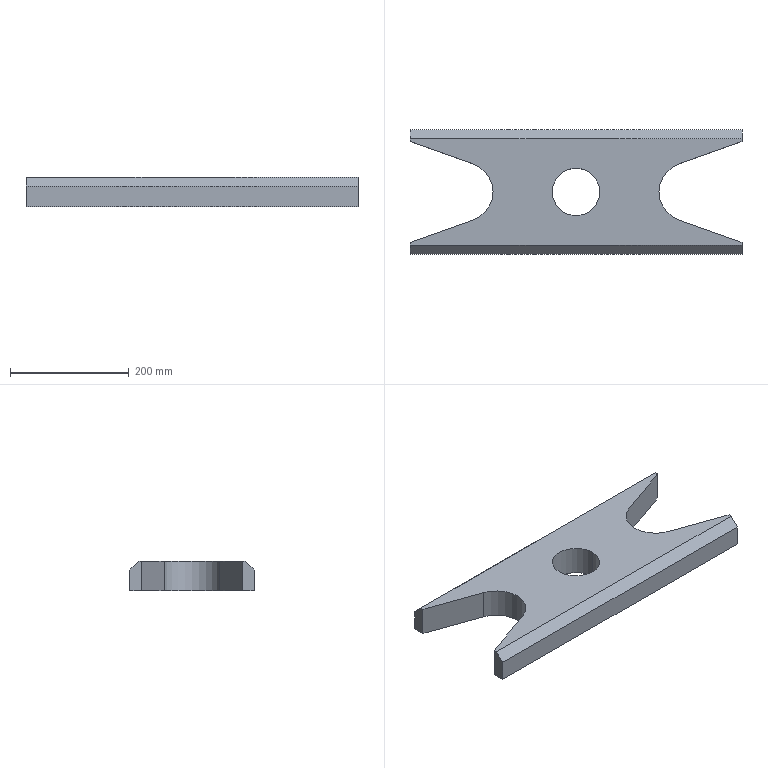Part | SolidWorks | features Chamfer 1, Extrusion 1 | 1 solid | 19 faces | box 560 x 210 x 50 mm | volume 3864002 mm3 | plane 14 | cylinder 5 | commonest cylinder face diameters 100 x3 80 x2
STEP:
#1=CARTESIAN_POINT('',(-40.,0.,25.));
#2=VERTEX_POINT('',#1);
#3=CARTESIAN_POINT('',(40.,0.,25.));
#4=VERTEX_POINT('',#3);
#5=CARTESIAN_POINT('',(0.,0.,25.));
#6=DIRECTION('',(0.,0.,1.));
#7=DIRECTION('',(1.,0.,0.));
#8=AXIS2_PLACEMENT_3D('',#5,#6,#7);
#9=CIRCLE('',#8,40.);
#10=EDGE_CURVE('',#2,#4,#9,.T.);
#11=ORIENTED_EDGE('',*,*,#10,.T.);
#12=CARTESIAN_POINT('',(40.,0.,-25.));
#13=VERTEX_POINT('',#12);
#14=CARTESIAN_POINT('',(40.,0.,25.));
#15=DIRECTION('',(0.,0.,-1.));
#16=VECTOR('',#15,1000.);
#17=LINE('',#14,#16);
#18=EDGE_CURVE('',#4,#13,#17,.T.);
#19=ORIENTED_EDGE('',*,*,#18,.T.);
#20=CARTESIAN_POINT('',(-40.,0.,-25.));
#21=VERTEX_POINT('',#20);
#22=CARTESIAN_POINT('',(0.,0.,-25.));
#23=DIRECTION('',(0.,0.,1.));
#24=DIRECTION('',(1.,0.,0.));
#25=AXIS2_PLACEMENT_3D('',#22,#23,#24);
#26=CIRCLE('',#25,40.);
#27=EDGE_CURVE('',#21,#13,#26,.T.);
#28=ORIENTED_EDGE('',*,*,#27,.F.);
#29=CARTESIAN_POINT('',(-40.,0.,25.));
#30=DIRECTION('',(0.,0.,-1.));
#31=VECTOR('',#30,1000.);
#32=LINE('',#29,#31);
#33=EDGE_CURVE('',#2,#21,#32,.T.);
#34=ORIENTED_EDGE('',*,*,#33,.F.);
#35=EDGE_LOOP('',(#11,#19,#28,#34));
#36=FACE_OUTER_BOUND('',#35,.T.);
#37=CARTESIAN_POINT('',(0.,0.,25.));
#38=DIRECTION('',(0.,0.,-1.));
#39=DIRECTION('',(-1.,0.,0.));
#40=AXIS2_PLACEMENT_3D('',#37,#38,#39);
#41=CYLINDRICAL_SURFACE('',#40,40.);
#42=ADVANCED_FACE('',(#36),#41,.F.);
#43=CARTESIAN_POINT('',(140.,0.,25.));
#44=VERTEX_POINT('',#43);
#45=CARTESIAN_POINT('',(173.276,47.12,25.));
#46=VERTEX_POINT('',#45);
#47=CARTESIAN_POINT('',(190.,0.,25.));
#48=DIRECTION('',(0.,0.,-1.));
#49=DIRECTION('',(1.,0.,0.));
#50=AXIS2_PLACEMENT_3D('',#47,#48,#49);
#51=CIRCLE('',#50,50.);
#52=EDGE_CURVE('',#44,#46,#51,.T.);
#53=ORIENTED_EDGE('',*,*,#52,.F.);
#54=CARTESIAN_POINT('',(140.,0.,-25.));
#55=VERTEX_POINT('',#54);
#56=CARTESIAN_POINT('',(140.,0.,25.));
#57=DIRECTION('',(0.,0.,-1.));
#58=VECTOR('',#57,1000.);
#59=LINE('',#56,#58);
#60=EDGE_CURVE('',#44,#55,#59,.T.);
#61=ORIENTED_EDGE('',*,*,#60,.T.);
#62=CARTESIAN_POINT('',(173.276,47.12,-25.));
#63=VERTEX_POINT('',#62);
#64=CARTESIAN_POINT('',(190.,0.,-25.));
#65=DIRECTION('',(0.,0.,-1.));
#66=DIRECTION('',(1.,0.,0.));
#67=AXIS2_PLACEMENT_3D('',#64,#65,#66);
#68=CIRCLE('',#67,50.);
#69=EDGE_CURVE('',#55,#63,#68,.T.);
#70=ORIENTED_EDGE('',*,*,#69,.T.);
#71=CARTESIAN_POINT('',(173.276,47.12,25.));
#72=DIRECTION('',(0.,0.,-1.));
#73=VECTOR('',#72,1000.);
#74=LINE('',#71,#73);
#75=EDGE_CURVE('',#46,#63,#74,.T.);
#76=ORIENTED_EDGE('',*,*,#75,.F.);
#77=EDGE_LOOP('',(#53,#61,#70,#76));
#78=FACE_OUTER_BOUND('',#77,.T.);
#79=CARTESIAN_POINT('',(190.,0.,25.));
#80=DIRECTION('',(0.,0.,-1.));
#81=DIRECTION('',(-1.,0.,0.));
#82=AXIS2_PLACEMENT_3D('',#79,#80,#81);
#83=CYLINDRICAL_SURFACE('',#82,50.);
#84=ADVANCED_FACE('',(#78),#83,.F.);
#85=CARTESIAN_POINT('',(-280.,-85.,25.));
#86=VERTEX_POINT('',#85);
#87=CARTESIAN_POINT('',(-280.,-90.,25.));
#88=VERTEX_POINT('',#87);
#89=CARTESIAN_POINT('',(-280.,-105.,25.));
#90=DIRECTION('',(0.,-1.,0.));
#91=VECTOR('',#90,1000.);
#92=LINE('',#89,#91);
#93=EDGE_CURVE('',#86,#88,#92,.T.);
#94=ORIENTED_EDGE('',*,*,#93,.T.);
#95=CARTESIAN_POINT('',(280.,-90.,25.));
#96=VERTEX_POINT('',#95);
#97=CARTESIAN_POINT('',(280.,-90.,25.));
#98=DIRECTION('',(1.,0.,0.));
#99=VECTOR('',#98,1000.);
#100=LINE('',#97,#99);
#101=EDGE_CURVE('',#88,#96,#100,.T.);
#102=ORIENTED_EDGE('',*,*,#101,.T.);
#103=CARTESIAN_POINT('',(280.,-85.,25.));
#104=VERTEX_POINT('',#103);
#105=CARTESIAN_POINT('',(280.,-105.,25.));
#106=DIRECTION('',(0.,1.,0.));
#107=VECTOR('',#106,1000.);
#108=LINE('',#105,#107);
#109=EDGE_CURVE('',#96,#104,#108,.T.);
#110=ORIENTED_EDGE('',*,*,#109,.T.);
#111=CARTESIAN_POINT('',(173.276,-47.12,25.));
#112=VERTEX_POINT('',#111);
#113=CARTESIAN_POINT('',(280.,-85.,25.));
#114=DIRECTION('',(-0.9424,0.3345,0.));
#115=VECTOR('',#114,1000.);
#116=LINE('',#113,#115);
#117=EDGE_CURVE('',#104,#112,#116,.T.);
#118=ORIENTED_EDGE('',*,*,#117,.T.);
#119=CARTESIAN_POINT('',(190.,0.,25.));
#120=DIRECTION('',(0.,0.,-1.));
#121=DIRECTION('',(1.,0.,0.));
#122=AXIS2_PLACEMENT_3D('',#119,#120,#121);
#123=CIRCLE('',#122,50.);
#124=EDGE_CURVE('',#112,#44,#123,.T.);
#125=ORIENTED_EDGE('',*,*,#124,.T.);
#126=ORIENTED_EDGE('',*,*,#52,.T.);
#127=CARTESIAN_POINT('',(280.,85.,25.));
#128=VERTEX_POINT('',#127);
#129=CARTESIAN_POINT('',(280.,85.,25.));
#130=DIRECTION('',(0.9424,0.3345,0.));
#131=VECTOR('',#130,1000.);
#132=LINE('',#129,#131);
#133=EDGE_CURVE('',#46,#128,#132,.T.);
#134=ORIENTED_EDGE('',*,*,#133,.T.);
#135=CARTESIAN_POINT('',(280.,90.,25.));
#136=VERTEX_POINT('',#135);
#137=CARTESIAN_POINT('',(280.,105.,25.));
#138=DIRECTION('',(0.,1.,0.));
#139=VECTOR('',#138,1000.);
#140=LINE('',#137,#139);
#141=EDGE_CURVE('',#128,#136,#140,.T.);
#142=ORIENTED_EDGE('',*,*,#141,.T.);
#143=CARTESIAN_POINT('',(-280.,90.,25.));
#144=VERTEX_POINT('',#143);
#145=CARTESIAN_POINT('',(-280.,90.,25.));
#146=DIRECTION('',(-1.,0.,0.));
#147=VECTOR('',#146,1000.);
#148=LINE('',#145,#147);
#149=EDGE_CURVE('',#136,#144,#148,.T.);
#150=ORIENTED_EDGE('',*,*,#149,.T.);
#151=CARTESIAN_POINT('',(-280.,85.,25.));
#152=VERTEX_POINT('',#151);
#153=CARTESIAN_POINT('',(-280.,105.,25.));
#154=DIRECTION('',(0.,-1.,0.));
#155=VECTOR('',#154,1000.);
#156=LINE('',#153,#155);
#157=EDGE_CURVE('',#144,#152,#156,.T.);
#158=ORIENTED_EDGE('',*,*,#157,.T.);
#159=CARTESIAN_POINT('',(-173.276,47.12,25.));
#160=VERTEX_POINT('',#159);
#161=CARTESIAN_POINT('',(-280.,85.,25.));
#162=DIRECTION('',(0.9424,-0.3345,0.));
#163=VECTOR('',#162,1000.);
#164=LINE('',#161,#163);
#165=EDGE_CURVE('',#152,#160,#164,.T.);
#166=ORIENTED_EDGE('',*,*,#165,.T.);
#167=CARTESIAN_POINT('',(-173.276,-47.12,25.));
#168=VERTEX_POINT('',#167);
#169=CARTESIAN_POINT('',(-190.,0.,25.));
#170=DIRECTION('',(0.,0.,-1.));
#171=DIRECTION('',(-1.,0.,0.));
#172=AXIS2_PLACEMENT_3D('',#169,#170,#171);
#173=CIRCLE('',#172,50.);
#174=EDGE_CURVE('',#160,#168,#173,.T.);
#175=ORIENTED_EDGE('',*,*,#174,.T.);
#176=CARTESIAN_POINT('',(-280.,-85.,25.));
#177=DIRECTION('',(-0.9424,-0.3345,0.));
#178=VECTOR('',#177,1000.);
#179=LINE('',#176,#178);
#180=EDGE_CURVE('',#168,#86,#179,.T.);
#181=ORIENTED_EDGE('',*,*,#180,.T.);
#182=EDGE_LOOP('',(#94,#102,#110,#118,#125,#126,#134,#142,#150,#158,#166,#175,#181));
#183=FACE_OUTER_BOUND('',#182,.T.);
#184=ORIENTED_EDGE('',*,*,#10,.F.);
#185=CARTESIAN_POINT('',(0.,0.,25.));
#186=DIRECTION('',(0.,0.,1.));
#187=DIRECTION('',(1.,0.,0.));
#188=AXIS2_PLACEMENT_3D('',#185,#186,#187);
#189=CIRCLE('',#188,40.);
#190=EDGE_CURVE('',#4,#2,#189,.T.);
#191=ORIENTED_EDGE('',*,*,#190,.F.);
#192=EDGE_LOOP('',(#184,#191));
#193=FACE_BOUND('',#192,.T.);
#194=CARTESIAN_POINT('',(190.,0.,25.));
#195=DIRECTION('',(0.,0.,1.));
#196=DIRECTION('',(1.,0.,0.));
#197=AXIS2_PLACEMENT_3D('',#194,#195,#196);
#198=PLANE('',#197);
#199=ADVANCED_FACE('',(#183,#193),#198,.T.);
#200=CARTESIAN_POINT('',(280.,85.,-25.));
#201=VERTEX_POINT('',#200);
#202=CARTESIAN_POINT('',(280.,85.,-25.));
#203=DIRECTION('',(0.9424,0.3345,0.));
#204=VECTOR('',#203,1000.);
#205=LINE('',#202,#204);
#206=EDGE_CURVE('',#63,#201,#205,.T.);
#207=ORIENTED_EDGE('',*,*,#206,.F.);
#208=ORIENTED_EDGE('',*,*,#69,.F.);
#209=CARTESIAN_POINT('',(173.276,-47.12,-25.));
#210=VERTEX_POINT('',#209);
#211=CARTESIAN_POINT('',(190.,0.,-25.));
#212=DIRECTION('',(0.,0.,-1.));
#213=DIRECTION('',(1.,0.,0.));
#214=AXIS2_PLACEMENT_3D('',#211,#212,#213);
#215=CIRCLE('',#214,50.);
#216=EDGE_CURVE('',#210,#55,#215,.T.);
#217=ORIENTED_EDGE('',*,*,#216,.F.);
#218=CARTESIAN_POINT('',(280.,-85.,-25.));
#219=VERTEX_POINT('',#218);
#220=CARTESIAN_POINT('',(280.,-85.,-25.));
#221=DIRECTION('',(-0.9424,0.3345,0.));
#222=VECTOR('',#221,1000.);
#223=LINE('',#220,#222);
#224=EDGE_CURVE('',#219,#210,#223,.T.);
#225=ORIENTED_EDGE('',*,*,#224,.F.);
#226=CARTESIAN_POINT('',(280.,-105.,-25.));
#227=VERTEX_POINT('',#226);
#228=CARTESIAN_POINT('',(280.,-105.,-25.));
#229=DIRECTION('',(0.,1.,0.));
#230=VECTOR('',#229,1000.);
#231=LINE('',#228,#230);
#232=EDGE_CURVE('',#227,#219,#231,.T.);
#233=ORIENTED_EDGE('',*,*,#232,.F.);
#234=CARTESIAN_POINT('',(-280.,-105.,-25.));
#235=VERTEX_POINT('',#234);
#236=CARTESIAN_POINT('',(-280.,-105.,-25.));
#237=DIRECTION('',(1.,0.,0.));
#238=VECTOR('',#237,1000.);
#239=LINE('',#236,#238);
#240=EDGE_CURVE('',#235,#227,#239,.T.);
#241=ORIENTED_EDGE('',*,*,#240,.F.);
#242=CARTESIAN_POINT('',(-280.,-85.,-25.));
#243=VERTEX_POINT('',#242);
#244=CARTESIAN_POINT('',(-280.,-105.,-25.));
#245=DIRECTION('',(0.,-1.,0.));
#246=VECTOR('',#245,1000.);
#247=LINE('',#244,#246);
#248=EDGE_CURVE('',#243,#235,#247,.T.);
#249=ORIENTED_EDGE('',*,*,#248,.F.);
#250=CARTESIAN_POINT('',(-173.276,-47.12,-25.));
#251=VERTEX_POINT('',#250);
#252=CARTESIAN_POINT('',(-280.,-85.,-25.));
#253=DIRECTION('',(-0.9424,-0.3345,0.));
#254=VECTOR('',#253,1000.);
#255=LINE('',#252,#254);
#256=EDGE_CURVE('',#251,#243,#255,.T.);
#257=ORIENTED_EDGE('',*,*,#256,.F.);
#258=CARTESIAN_POINT('',(-173.276,47.12,-25.));
#259=VERTEX_POINT('',#258);
#260=CARTESIAN_POINT('',(-190.,0.,-25.));
#261=DIRECTION('',(0.,0.,-1.));
#262=DIRECTION('',(-1.,0.,0.));
#263=AXIS2_PLACEMENT_3D('',#260,#261,#262);
#264=CIRCLE('',#263,50.);
#265=EDGE_CURVE('',#259,#251,#264,.T.);
#266=ORIENTED_EDGE('',*,*,#265,.F.);
#267=CARTESIAN_POINT('',(-280.,85.,-25.));
#268=VERTEX_POINT('',#267);
#269=CARTESIAN_POINT('',(-280.,85.,-25.));
#270=DIRECTION('',(0.9424,-0.3345,0.));
#271=VECTOR('',#270,1000.);
#272=LINE('',#269,#271);
#273=EDGE_CURVE('',#268,#259,#272,.T.);
#274=ORIENTED_EDGE('',*,*,#273,.F.);
#275=CARTESIAN_POINT('',(-280.,105.,-25.));
#276=VERTEX_POINT('',#275);
#277=CARTESIAN_POINT('',(-280.,105.,-25.));
#278=DIRECTION('',(0.,-1.,0.));
#279=VECTOR('',#278,1000.);
#280=LINE('',#277,#279);
#281=EDGE_CURVE('',#276,#268,#280,.T.);
#282=ORIENTED_EDGE('',*,*,#281,.F.);
#283=CARTESIAN_POINT('',(280.,105.,-25.));
#284=VERTEX_POINT('',#283);
#285=CARTESIAN_POINT('',(-280.,105.,-25.));
#286=DIRECTION('',(-1.,0.,0.));
#287=VECTOR('',#286,1000.);
#288=LINE('',#285,#287);
#289=EDGE_CURVE('',#284,#276,#288,.T.);
#290=ORIENTED_EDGE('',*,*,#289,.F.);
#291=CARTESIAN_POINT('',(280.,105.,-25.));
#292=DIRECTION('',(0.,1.,0.));
#293=VECTOR('',#292,1000.);
#294=LINE('',#291,#293);
#295=EDGE_CURVE('',#201,#284,#294,.T.);
#296=ORIENTED_EDGE('',*,*,#295,.F.);
#297=EDGE_LOOP('',(#207,#208,#217,#225,#233,#241,#249,#257,#266,#274,#282,#290,#296));
#298=FACE_OUTER_BOUND('',#297,.T.);
#299=ORIENTED_EDGE('',*,*,#27,.T.);
#300=CARTESIAN_POINT('',(0.,0.,-25.));
#301=DIRECTION('',(0.,0.,1.));
#302=DIRECTION('',(1.,0.,0.));
#303=AXIS2_PLACEMENT_3D('',#300,#301,#302);
#304=CIRCLE('',#303,40.);
#305=EDGE_CURVE('',#13,#21,#304,.T.);
#306=ORIENTED_EDGE('',*,*,#305,.T.);
#307=EDGE_LOOP('',(#299,#306));
#308=FACE_BOUND('',#307,.T.);
#309=CARTESIAN_POINT('',(190.,0.,-25.));
#310=DIRECTION('',(0.,0.,1.));
#311=DIRECTION('',(1.,0.,0.));
#312=AXIS2_PLACEMENT_3D('',#309,#310,#311);
#313=PLANE('',#312);
#314=ADVANCED_FACE('',(#298,#308),#313,.F.);
#315=ORIENTED_EDGE('',*,*,#206,.T.);
#316=CARTESIAN_POINT('',(280.,85.,25.));
#317=DIRECTION('',(0.,0.,-1.));
#318=VECTOR('',#317,1000.);
#319=LINE('',#316,#318);
#320=EDGE_CURVE('',#128,#201,#319,.T.);
#321=ORIENTED_EDGE('',*,*,#320,.F.);
#322=ORIENTED_EDGE('',*,*,#133,.F.);
#323=ORIENTED_EDGE('',*,*,#75,.T.);
#324=EDGE_LOOP('',(#315,#321,#322,#323));
#325=FACE_OUTER_BOUND('',#324,.T.);
#326=CARTESIAN_POINT('',(280.,85.,25.));
#327=DIRECTION('',(-0.3345,0.9424,0.));
#328=DIRECTION('',(-0.9424,-0.3345,0.));
#329=AXIS2_PLACEMENT_3D('',#326,#327,#328);
#330=PLANE('',#329);
#331=ADVANCED_FACE('',(#325),#330,.F.);
#332=CARTESIAN_POINT('',(280.,105.,10.));
#333=VERTEX_POINT('',#332);
#334=CARTESIAN_POINT('',(280.,105.,25.));
#335=DIRECTION('',(0.,0.,-1.));
#336=VECTOR('',#335,1000.);
#337=LINE('',#334,#336);
#338=EDGE_CURVE('',#333,#284,#337,.T.);
#339=ORIENTED_EDGE('',*,*,#338,.F.);
#340=CARTESIAN_POINT('',(280.,90.,25.));
#341=DIRECTION('',(0.,-0.7071,0.7071));
#342=VECTOR('',#341,1000.);
#343=LINE('',#340,#342);
#344=EDGE_CURVE('',#333,#136,#343,.T.);
#345=ORIENTED_EDGE('',*,*,#344,.T.);
#346=ORIENTED_EDGE('',*,*,#141,.F.);
#347=ORIENTED_EDGE('',*,*,#320,.T.);
#348=ORIENTED_EDGE('',*,*,#295,.T.);
#349=EDGE_LOOP('',(#339,#345,#346,#347,#348));
#350=FACE_OUTER_BOUND('',#349,.T.);
#351=CARTESIAN_POINT('',(280.,105.,25.));
#352=DIRECTION('',(-1.,0.,0.));
#353=DIRECTION('',(0.,-1.,0.));
#354=AXIS2_PLACEMENT_3D('',#351,#352,#353);
#355=PLANE('',#354);
#356=ADVANCED_FACE('',(#350),#355,.F.);
#357=CARTESIAN_POINT('',(-280.,105.,10.));
#358=VERTEX_POINT('',#357);
#359=CARTESIAN_POINT('',(-280.,105.,25.));
#360=DIRECTION('',(0.,0.,-1.));
#361=VECTOR('',#360,1000.);
#362=LINE('',#359,#361);
#363=EDGE_CURVE('',#358,#276,#362,.T.);
#364=ORIENTED_EDGE('',*,*,#363,.F.);
#365=CARTESIAN_POINT('',(280.,105.,10.));
#366=DIRECTION('',(1.,0.,0.));
#367=VECTOR('',#366,1000.);
#368=LINE('',#365,#367);
#369=EDGE_CURVE('',#358,#333,#368,.T.);
#370=ORIENTED_EDGE('',*,*,#369,.T.);
#371=ORIENTED_EDGE('',*,*,#338,.T.);
#372=ORIENTED_EDGE('',*,*,#289,.T.);
#373=EDGE_LOOP('',(#364,#370,#371,#372));
#374=FACE_OUTER_BOUND('',#373,.T.);
#375=CARTESIAN_POINT('',(-280.,105.,25.));
#376=DIRECTION('',(0.,-1.,0.));
#377=DIRECTION('',(0.,0.,-1.));
#378=AXIS2_PLACEMENT_3D('',#375,#376,#377);
#379=PLANE('',#378);
#380=ADVANCED_FACE('',(#374),#379,.F.);
#381=ORIENTED_EDGE('',*,*,#157,.F.);
#382=CARTESIAN_POINT('',(-280.,90.,25.));
#383=DIRECTION('',(0.,0.7071,-0.7071));
#384=VECTOR('',#383,1000.);
#385=LINE('',#382,#384);
#386=EDGE_CURVE('',#144,#358,#385,.T.);
#387=ORIENTED_EDGE('',*,*,#386,.T.);
#388=ORIENTED_EDGE('',*,*,#363,.T.);
#389=ORIENTED_EDGE('',*,*,#281,.T.);
#390=CARTESIAN_POINT('',(-280.,85.,25.));
#391=DIRECTION('',(0.,0.,-1.));
#392=VECTOR('',#391,1000.);
#393=LINE('',#390,#392);
#394=EDGE_CURVE('',#152,#268,#393,.T.);
#395=ORIENTED_EDGE('',*,*,#394,.F.);
#396=EDGE_LOOP('',(#381,#387,#388,#389,#395));
#397=FACE_OUTER_BOUND('',#396,.T.);
#398=CARTESIAN_POINT('',(-280.,105.,25.));
#399=DIRECTION('',(1.,0.,0.));
#400=DIRECTION('',(0.,1.,0.));
#401=AXIS2_PLACEMENT_3D('',#398,#399,#400);
#402=PLANE('',#401);
#403=ADVANCED_FACE('',(#397),#402,.F.);
#404=ORIENTED_EDGE('',*,*,#273,.T.);
#405=CARTESIAN_POINT('',(-173.276,47.12,25.));
#406=DIRECTION('',(0.,0.,-1.));
#407=VECTOR('',#406,1000.);
#408=LINE('',#405,#407);
#409=EDGE_CURVE('',#160,#259,#408,.T.);
#410=ORIENTED_EDGE('',*,*,#409,.F.);
#411=ORIENTED_EDGE('',*,*,#165,.F.);
#412=ORIENTED_EDGE('',*,*,#394,.T.);
#413=EDGE_LOOP('',(#404,#410,#411,#412));
#414=FACE_OUTER_BOUND('',#413,.T.);
#415=CARTESIAN_POINT('',(-280.,85.,25.));
#416=DIRECTION('',(0.3345,0.9424,0.));
#417=DIRECTION('',(-0.9424,0.3345,0.));
#418=AXIS2_PLACEMENT_3D('',#415,#416,#417);
#419=PLANE('',#418);
#420=ADVANCED_FACE('',(#414),#419,.F.);
#421=ORIENTED_EDGE('',*,*,#265,.T.);
#422=CARTESIAN_POINT('',(-173.276,-47.12,25.));
#423=DIRECTION('',(0.,0.,-1.));
#424=VECTOR('',#423,1000.);
#425=LINE('',#422,#424);
#426=EDGE_CURVE('',#168,#251,#425,.T.);
#427=ORIENTED_EDGE('',*,*,#426,.F.);
#428=ORIENTED_EDGE('',*,*,#174,.F.);
#429=ORIENTED_EDGE('',*,*,#409,.T.);
#430=EDGE_LOOP('',(#421,#427,#428,#429));
#431=FACE_OUTER_BOUND('',#430,.T.);
#432=CARTESIAN_POINT('',(-190.,0.,25.));
#433=DIRECTION('',(0.,0.,-1.));
#434=DIRECTION('',(-1.,0.,0.));
#435=AXIS2_PLACEMENT_3D('',#432,#433,#434);
#436=CYLINDRICAL_SURFACE('',#435,50.);
#437=ADVANCED_FACE('',(#431),#436,.F.);
#438=ORIENTED_EDGE('',*,*,#256,.T.);
#439=CARTESIAN_POINT('',(-280.,-85.,25.));
#440=DIRECTION('',(0.,0.,-1.));
#441=VECTOR('',#440,1000.);
#442=LINE('',#439,#441);
#443=EDGE_CURVE('',#86,#243,#442,.T.);
#444=ORIENTED_EDGE('',*,*,#443,.F.);
#445=ORIENTED_EDGE('',*,*,#180,.F.);
#446=ORIENTED_EDGE('',*,*,#426,.T.);
#447=EDGE_LOOP('',(#438,#444,#445,#446));
#448=FACE_OUTER_BOUND('',#447,.T.);
#449=CARTESIAN_POINT('',(-280.,-85.,25.));
#450=DIRECTION('',(0.3345,-0.9424,0.));
#451=DIRECTION('',(0.9424,0.3345,0.));
#452=AXIS2_PLACEMENT_3D('',#449,#450,#451);
#453=PLANE('',#452);
#454=ADVANCED_FACE('',(#448),#453,.F.);
#455=CARTESIAN_POINT('',(-280.,-105.,10.));
#456=VERTEX_POINT('',#455);
#457=CARTESIAN_POINT('',(-280.,-105.,25.));
#458=DIRECTION('',(0.,0.,-1.));
#459=VECTOR('',#458,1000.);
#460=LINE('',#457,#459);
#461=EDGE_CURVE('',#456,#235,#460,.T.);
#462=ORIENTED_EDGE('',*,*,#461,.F.);
#463=CARTESIAN_POINT('',(-280.,-90.,25.));
#464=DIRECTION('',(0.,0.7071,0.7071));
#465=VECTOR('',#464,1000.);
#466=LINE('',#463,#465);
#467=EDGE_CURVE('',#456,#88,#466,.T.);
#468=ORIENTED_EDGE('',*,*,#467,.T.);
#469=ORIENTED_EDGE('',*,*,#93,.F.);
#470=ORIENTED_EDGE('',*,*,#443,.T.);
#471=ORIENTED_EDGE('',*,*,#248,.T.);
#472=EDGE_LOOP('',(#462,#468,#469,#470,#471));
#473=FACE_OUTER_BOUND('',#472,.T.);
#474=CARTESIAN_POINT('',(-280.,-105.,25.));
#475=DIRECTION('',(1.,0.,0.));
#476=DIRECTION('',(0.,1.,0.));
#477=AXIS2_PLACEMENT_3D('',#474,#475,#476);
#478=PLANE('',#477);
#479=ADVANCED_FACE('',(#473),#478,.F.);
#480=CARTESIAN_POINT('',(280.,-105.,10.));
#481=VERTEX_POINT('',#480);
#482=CARTESIAN_POINT('',(280.,-105.,25.));
#483=DIRECTION('',(0.,0.,-1.));
#484=VECTOR('',#483,1000.);
#485=LINE('',#482,#484);
#486=EDGE_CURVE('',#481,#227,#485,.T.);
#487=ORIENTED_EDGE('',*,*,#486,.F.);
#488=CARTESIAN_POINT('',(-280.,-105.,10.));
#489=DIRECTION('',(-1.,0.,0.));
#490=VECTOR('',#489,1000.);
#491=LINE('',#488,#490);
#492=EDGE_CURVE('',#481,#456,#491,.T.);
#493=ORIENTED_EDGE('',*,*,#492,.T.);
#494=ORIENTED_EDGE('',*,*,#461,.T.);
#495=ORIENTED_EDGE('',*,*,#240,.T.);
#496=EDGE_LOOP('',(#487,#493,#494,#495));
#497=FACE_OUTER_BOUND('',#496,.T.);
#498=CARTESIAN_POINT('',(-280.,-105.,25.));
#499=DIRECTION('',(0.,1.,0.));
#500=DIRECTION('',(0.,0.,1.));
#501=AXIS2_PLACEMENT_3D('',#498,#499,#500);
#502=PLANE('',#501);
#503=ADVANCED_FACE('',(#497),#502,.F.);
#504=ORIENTED_EDGE('',*,*,#109,.F.);
#505=CARTESIAN_POINT('',(280.,-90.,25.));
#506=DIRECTION('',(0.,-0.7071,-0.7071));
#507=VECTOR('',#506,1000.);
#508=LINE('',#505,#507);
#509=EDGE_CURVE('',#96,#481,#508,.T.);
#510=ORIENTED_EDGE('',*,*,#509,.T.);
#511=ORIENTED_EDGE('',*,*,#486,.T.);
#512=ORIENTED_EDGE('',*,*,#232,.T.);
#513=CARTESIAN_POINT('',(280.,-85.,25.));
#514=DIRECTION('',(0.,0.,-1.));
#515=VECTOR('',#514,1000.);
#516=LINE('',#513,#515);
#517=EDGE_CURVE('',#104,#219,#516,.T.);
#518=ORIENTED_EDGE('',*,*,#517,.F.);
#519=EDGE_LOOP('',(#504,#510,#511,#512,#518));
#520=FACE_OUTER_BOUND('',#519,.T.);
#521=CARTESIAN_POINT('',(280.,-105.,25.));
#522=DIRECTION('',(-1.,0.,0.));
#523=DIRECTION('',(0.,-1.,0.));
#524=AXIS2_PLACEMENT_3D('',#521,#522,#523);
#525=PLANE('',#524);
#526=ADVANCED_FACE('',(#520),#525,.F.);
#527=ORIENTED_EDGE('',*,*,#224,.T.);
#528=CARTESIAN_POINT('',(173.276,-47.12,25.));
#529=DIRECTION('',(0.,0.,-1.));
#530=VECTOR('',#529,1000.);
#531=LINE('',#528,#530);
#532=EDGE_CURVE('',#112,#210,#531,.T.);
#533=ORIENTED_EDGE('',*,*,#532,.F.);
#534=ORIENTED_EDGE('',*,*,#117,.F.);
#535=ORIENTED_EDGE('',*,*,#517,.T.);
#536=EDGE_LOOP('',(#527,#533,#534,#535));
#537=FACE_OUTER_BOUND('',#536,.T.);
#538=CARTESIAN_POINT('',(280.,-85.,25.));
#539=DIRECTION('',(-0.3345,-0.9424,0.));
#540=DIRECTION('',(0.9424,-0.3345,0.));
#541=AXIS2_PLACEMENT_3D('',#538,#539,#540);
#542=PLANE('',#541);
#543=ADVANCED_FACE('',(#537),#542,.F.);
#544=ORIENTED_EDGE('',*,*,#60,.F.);
#545=ORIENTED_EDGE('',*,*,#124,.F.);
#546=ORIENTED_EDGE('',*,*,#532,.T.);
#547=ORIENTED_EDGE('',*,*,#216,.T.);
#548=EDGE_LOOP('',(#544,#545,#546,#547));
#549=FACE_OUTER_BOUND('',#548,.T.);
#550=CARTESIAN_POINT('',(190.,0.,25.));
#551=DIRECTION('',(0.,0.,-1.));
#552=DIRECTION('',(-1.,0.,0.));
#553=AXIS2_PLACEMENT_3D('',#550,#551,#552);
#554=CYLINDRICAL_SURFACE('',#553,50.);
#555=ADVANCED_FACE('',(#549),#554,.F.);
#556=ORIENTED_EDGE('',*,*,#18,.F.);
#557=ORIENTED_EDGE('',*,*,#190,.T.);
#558=ORIENTED_EDGE('',*,*,#33,.T.);
#559=ORIENTED_EDGE('',*,*,#305,.F.);
#560=EDGE_LOOP('',(#556,#557,#558,#559));
#561=FACE_OUTER_BOUND('',#560,.T.);
#562=CARTESIAN_POINT('',(0.,0.,25.));
#563=DIRECTION('',(0.,0.,-1.));
#564=DIRECTION('',(-1.,0.,0.));
#565=AXIS2_PLACEMENT_3D('',#562,#563,#564);
#566=CYLINDRICAL_SURFACE('',#565,40.);
#567=ADVANCED_FACE('',(#561),#566,.F.);
#568=ORIENTED_EDGE('',*,*,#467,.F.);
#569=ORIENTED_EDGE('',*,*,#492,.F.);
#570=ORIENTED_EDGE('',*,*,#509,.F.);
#571=ORIENTED_EDGE('',*,*,#101,.F.);
#572=EDGE_LOOP('',(#568,#569,#570,#571));
#573=FACE_OUTER_BOUND('',#572,.T.);
#574=CARTESIAN_POINT('',(190.,-90.,25.));
#575=DIRECTION('',(0.,-0.7071,0.7071));
#576=DIRECTION('',(-1.,0.,0.));
#577=AXIS2_PLACEMENT_3D('',#574,#575,#576);
#578=PLANE('',#577);
#579=ADVANCED_FACE('',(#573),#578,.T.);
#580=ORIENTED_EDGE('',*,*,#344,.F.);
#581=ORIENTED_EDGE('',*,*,#369,.F.);
#582=ORIENTED_EDGE('',*,*,#386,.F.);
#583=ORIENTED_EDGE('',*,*,#149,.F.);
#584=EDGE_LOOP('',(#580,#581,#582,#583));
#585=FACE_OUTER_BOUND('',#584,.T.);
#586=CARTESIAN_POINT('',(190.,90.,25.));
#587=DIRECTION('',(0.,0.7071,0.7071));
#588=DIRECTION('',(1.,0.,0.));
#589=AXIS2_PLACEMENT_3D('',#586,#587,#588);
#590=PLANE('',#589);
#591=ADVANCED_FACE('',(#585),#590,.T.);
#592=CLOSED_SHELL('',(#42,#84,#199,#314,#331,#356,#380,#403,#420,#437,#454,#479,#503,#526,#543,#555,#567,#579,#591));
#593=MANIFOLD_SOLID_BREP('',#592);
#594=CARTESIAN_POINT('',(0.,0.,0.));
#595=DIRECTION('',(0.,0.,1.));
#596=DIRECTION('',(1.,0.,0.));
#597=AXIS2_PLACEMENT_3D('',#594,#595,#596);
#598=(LENGTH_UNIT()NAMED_UNIT(*)SI_UNIT(.MILLI.,.METRE.));
#599=UNCERTAINTY_MEASURE_WITH_UNIT(LENGTH_MEASURE(0.00001),#598,'','');
#600=(NAMED_UNIT(*)PLANE_ANGLE_UNIT()SI_UNIT($,.RADIAN.));
#601=(NAMED_UNIT(*)SI_UNIT($,.STERADIAN.)SOLID_ANGLE_UNIT());
#602=(GEOMETRIC_REPRESENTATION_CONTEXT(3)GLOBAL_UNCERTAINTY_ASSIGNED_CONTEXT((#599))GLOBAL_UNIT_ASSIGNED_CONTEXT((#598,#600,#601))REPRESENTATION_CONTEXT('',''));
#603=ADVANCED_BREP_SHAPE_REPRESENTATION('',(#593,#597),#602);